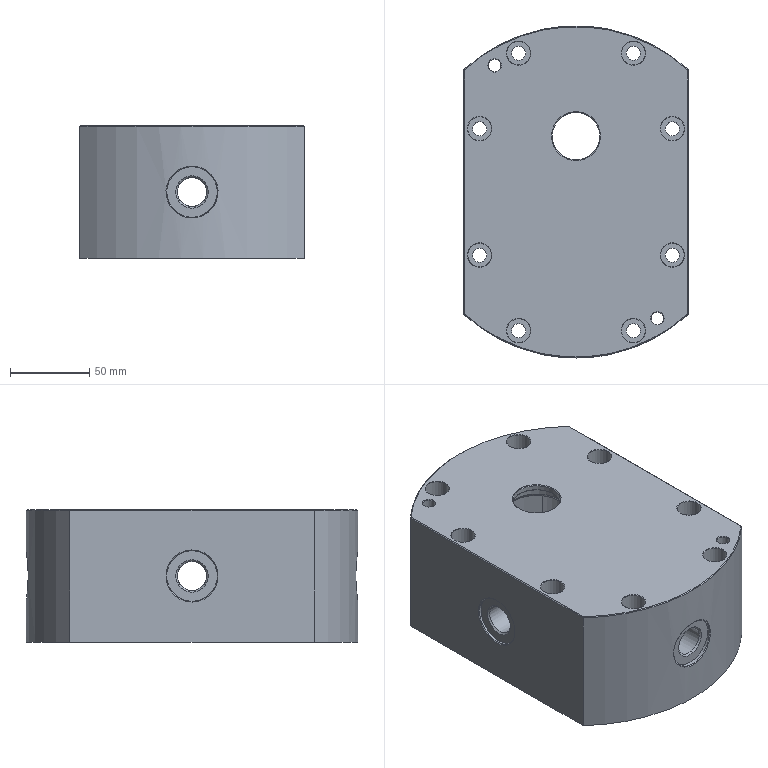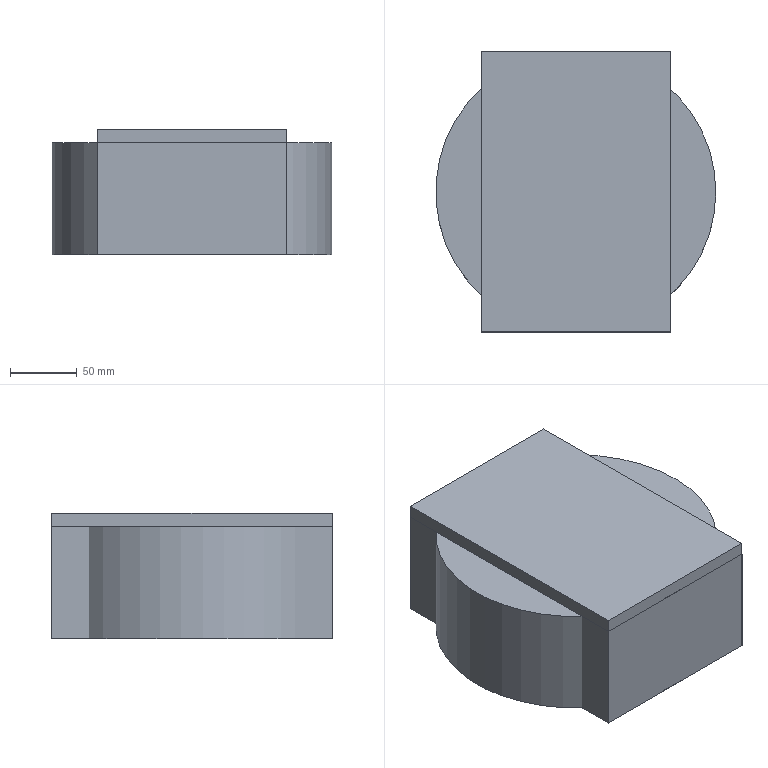CAM job | NX | 3+2 milling, drilling | part box 142 x 210 x 84 mm | stock box 210 x 210 x 94 mm
Tools:
number,name,description,diameter,corner_radius,flute_length,length,flutes
2,D50,Milling Tool-5 Parameters,50.0,0.0,50.0,75.0,2
10,D10,Milling Tool-5 Parameters,10.0,0.0,50.0,75.0,2
11,D10JING,Milling Tool-5 Parameters,10.0,0.0,50.0,75.0,2
7,D6A45,Milling Tool-5 Parameters,6.0,0.0,50.0,75.0,2
1,ZXZ,Milling Tool-5 Parameters,6.0,0.0,50.0,75.0,2
9,9.0ZT,Drilling Tool,9.0,0.0,35.0,50.0,2
8,7.8ZT,Drilling Tool,7.8,0.0,35.0,50.0,2
18,8.0JD,Milling Tool-5 Parameters,8.0,0.0,30.0,30.0,4
3,D3,Milling Tool-5 Parameters,3.0,0.0,50.0,75.0,2
5,D25R0.5,Milling Tool-5 Parameters,25.0,0.5,50.0,75.0,2
12,D12,Milling Tool-5 Parameters,12.0,0.0,50.0,75.0,2
Operations:
program,operation,operation_type,tool,method,geometry_group,spindle_rpm,surface_speed,feed_per_tooth,feed_cut,feed_plunge,cut_length_mm,path_length_mm,cut_time_min,machine_time_min
1,FLOOR_WALL,VolumeBased25DMillingOperation,D50,METHOD,A,1200.0,188.0,0.8333,2000.0,1000.0,78237.631,94862.018,39.41,41.072
1,FLOOR_WALL_COPY,VolumeBased25DMillingOperation,D50,METHOD,A,2500.0,392.0,0.2,1000.0,1000.0,994.848,1116.848,0.9948,1.007
1,HOLE_MILLING,CylinderMilling,D10,METHOD,A,3000.0,94.0,0.3667,2200.0,100.0,1761.999,1896.499,0.8009,0.8144
1,HOLE_MILLING_COPY,CylinderMilling,D10,METHOD,A,3000.0,94.0,0.3667,2200.0,100.0,2943.047,3098.547,1.338,1.353
1,HOLE_MILLING_COPY_1,CylinderMilling,D10JING,METHOD,A,5000.0,157.0,0.1,1000.0,100.0,95.013,227.013,0.095,0.1082
1,HOLE_MILLING_COPY_1_COPY,CylinderMilling,D10JING,METHOD,A,5000.0,157.0,0.1,1000.0,100.0,40.055,216.055,0.0401,0.0577
1,PLANAR_MILL,PlanarMilling,D6A45,METHOD,A,7500.0,141.0,0.0833,1250.0,100.0,436.87,994.544,0.3495,0.4053
1,PLANAR_MILL_COPY,PlanarMilling,D6A45,METHOD,A,7500.0,141.0,0.0833,1250.0,100.0,62.283,191.283,0.0498,0.0627
2,HOLE_MILLING_COPY_COPY,CylinderMilling,D10,METHOD,B,3000.0,94.0,0.3667,2200.0,100.0,20468.037,21671.752,9.304,9.424
2,HOLE_MILLING_COPY_COPY_COPY,CylinderMilling,D10,METHOD,B,3000.0,94.0,0.3667,2200.0,100.0,5441.462,5525.462,2.473,2.482
2,HOLE_MILLING_COPY_1_COPY_1,CylinderMilling,D10JING,METHOD,B,5000.0,157.0,0.1,1000.0,100.0,86.762,170.762,0.0868,0.0952
2,PLANAR_MILL_COPY_COPY,PlanarMilling,D6A45,METHOD,B,7500.0,141.0,0.0833,1250.0,100.0,498.26,1519.817,0.3986,0.5008
3,FLOOR_WALL_COPY_1,VolumeBased25DMillingOperation,D50,METHOD,C,1200.0,188.0,0.8333,2000.0,1000.0,45065.913,55289.613,22.62,23.642
3,FLOOR_WALL_COPY_COPY,VolumeBased25DMillingOperation,D50,METHOD,C,2500.0,392.0,0.2,1000.0,1000.0,1553.997,1607.997,1.554,1.559
3,DRILLING_COPY_1,Operation,ZXZ,METHOD,C,5000.0,94.0,0.025,250.0,0.0,40.0,617.281,0.16,0.2177
3,DRILLING_COPY,Operation,9.0ZT,METHOD,C,2000.0,56.0,0.0375,150.0,0.0,449.631,1421.202,2.998,3.095
3,DRILLING_COPY_COPY,Operation,7.8ZT,METHOD,C,2000.0,56.0,0.0375,150.0,0.0,52.687,358.684,0.3512,0.3818
3,DRILLING_COPY_COPY_COPY,Operation,8.0JD,METHOD,C,800.0,20.0,0.0125,40.0,0.0,46.0,345.31,1.15,1.18
3,PLANAR_PROFILE,PlanarMilling,D3,METHOD,C,5000.0,47.0,0.11,1100.0,500.0,18235.796,18291.596,16.698,16.703
3,FLOOR_WALL_1,VolumeBased25DMillingOperation,D25R0.5,METHOD,C,2000.0,157.0,0.55,2200.0,1000.0,189978.625,197879.838,94.291,95.081
3,HOLE_MILLING_COPY_COPY_COPY_COPY,CylinderMilling,D12,METHOD,C,3000.0,113.0,0.25,1500.0,100.0,3488.017,3699.517,2.325,2.346
3,FLOOR_WALL_1_COPY,VolumeBased25DMillingOperation,D12,METHOD,C,4000.0,150.0,0.125,1000.0,500.0,3595.242,3802.516,3.658,3.679
3,FLOOR_WALL_1_COPY_COPY,VolumeBased25DMillingOperation,D12,METHOD,C,4000.0,150.0,0.125,1000.0,500.0,2822.067,3020.067,2.828,2.847
3,PLANAR_MILL_COPY_COPY_COPY,PlanarMilling,D6A45,METHOD,C,7500.0,141.0,0.0833,1250.0,100.0,2397.747,3677.903,1.918,2.046
3,CUTTERCOMP12,CylinderMilling,D12,METHOD,C,4000.0,150.0,0.125,1000.0,100.0,98.453,318.453,0.0985,0.1205
4,HOLE_MILLING_COPY_2,CylinderMilling,D10,METHOD,D,3000.0,94.0,0.3667,2200.0,100.0,2468.241,2537.875,1.122,1.129
4,HOLE_MILLING_COPY_COPY_1,CylinderMilling,D10,METHOD,D,3000.0,94.0,0.3667,2200.0,100.0,2587.464,2673.964,1.176,1.185
4,HOLE_MILLING_COPY_1_COPY_2,CylinderMilling,D10JING,METHOD,D,5000.0,157.0,0.1,1000.0,100.0,95.013,161.013,0.095,0.1016
4,HOLE_MILLING_COPY_1_COPY_COPY,CylinderMilling,D10JING,METHOD,D,5000.0,157.0,0.1,1000.0,100.0,39.296,147.296,0.0393,0.0501
4,PLANAR_MILL_COPY_COPY_COPY_1,PlanarMilling,D6A45,METHOD,D,7500.0,141.0,0.0833,1250.0,100.0,65.383,128.383,0.0523,0.0586
4,PROFILE_3D,PlanarMilling,D6A45,METHOD,D,7500.0,141.0,0.0833,1250.0,100.0,106.912,162.955,0.0855,0.0911